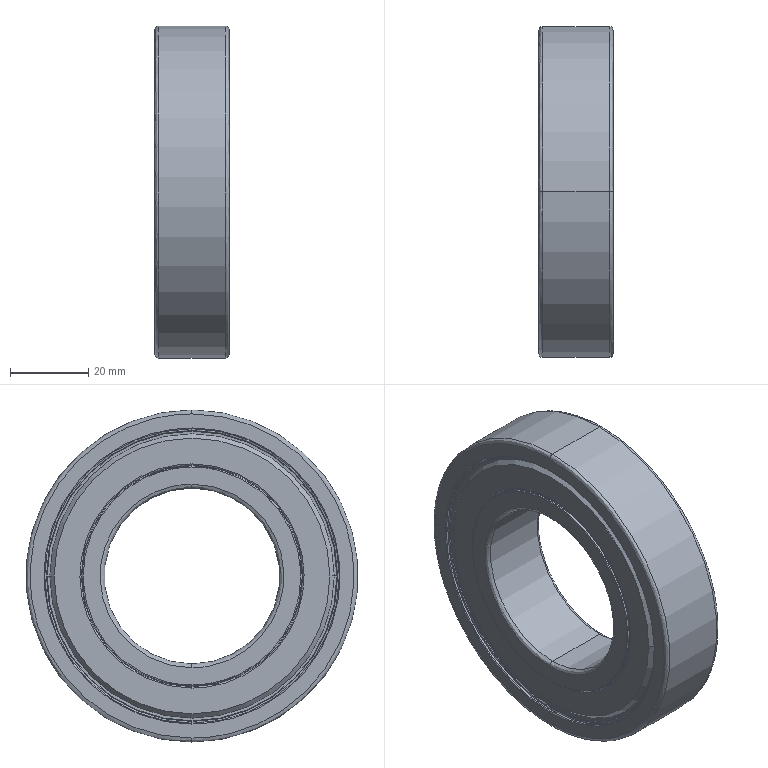Part | SolidWorks | features BaseBody 1 | 1 solid | 136 faces | box 19 x 85 x 85 mm | volume 65838 mm3 | spline 56 | cone 40 | cylinder 28 | plane 12 | commonest cylinder face diameters 56.2 x4 56.8 x4 57.4 x4 57.8 x4 73.2 x4 75.4 x4